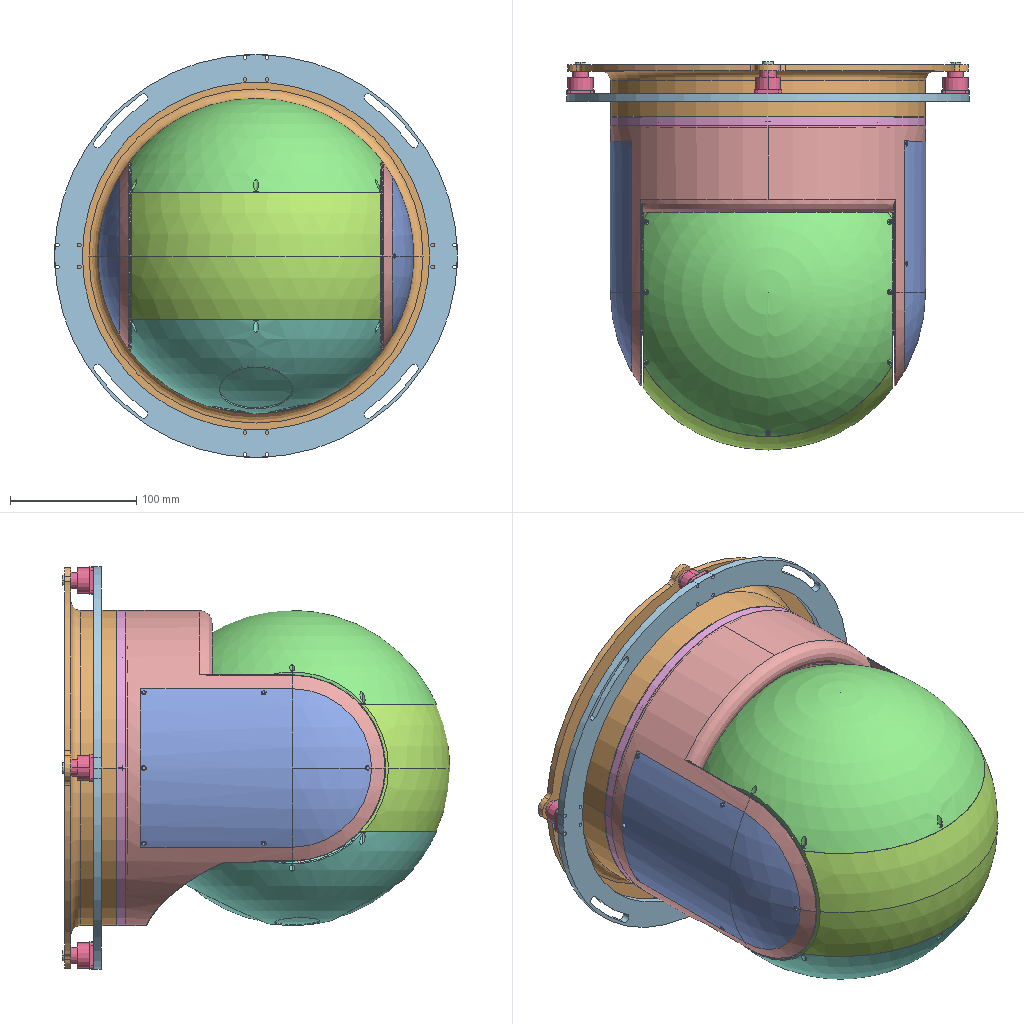Assembly | SolidWorks | 31 different items | 42 placed | box 319 x 308 x 319 mm
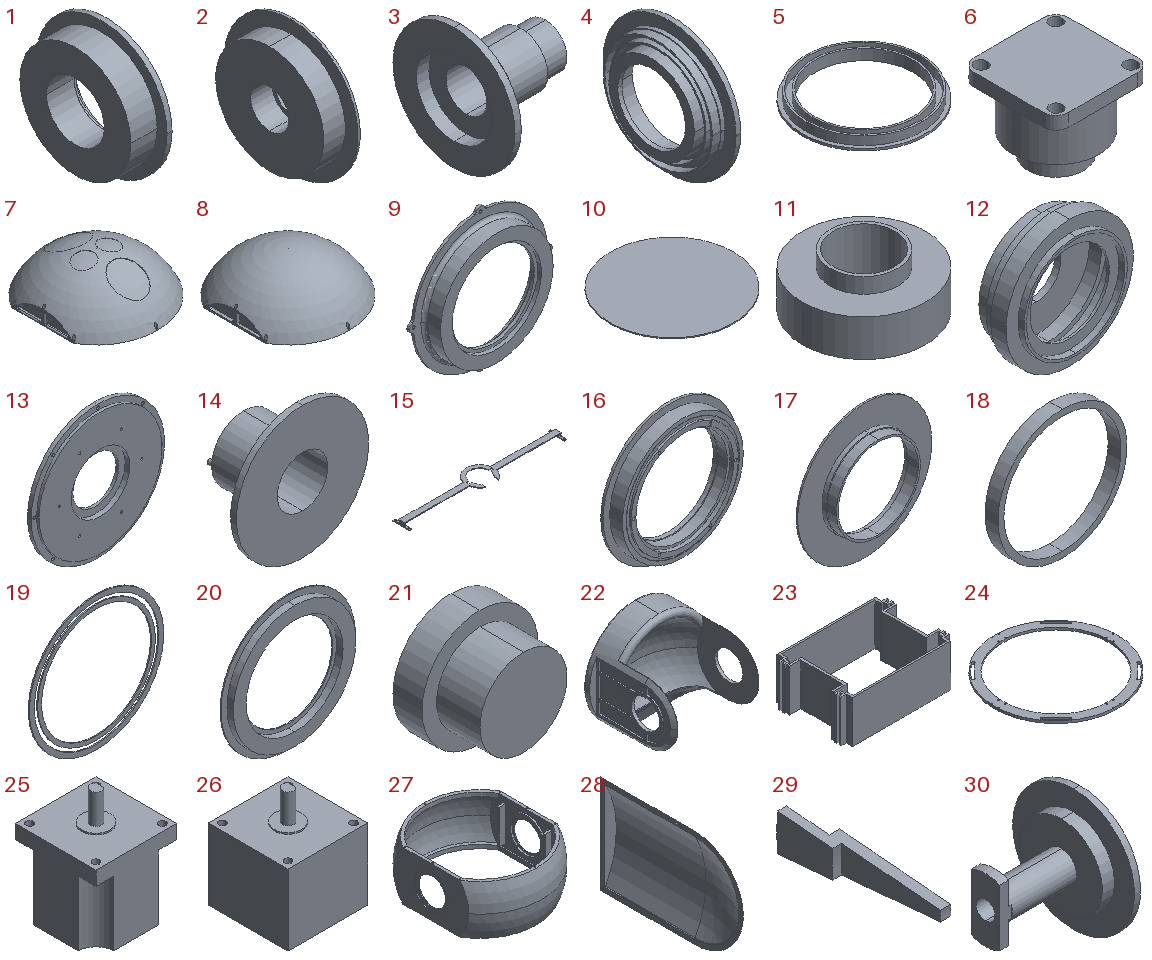Parts list (item | quantity | size | volume | features):
1 | x2 | 21.418 x 78.909 x 78.909 mm | 50880 mm3 | features Revolution 1
2 | x1 | 11.085 x 60.752 x 60.752 mm | 17812 mm3 | features Revolution 1
3 | x1 | 36.357 x 48.558 x 48.558 mm | 9786 mm3 | features Revolution 1
4 | x2 | 14.383 x 84 x 84 mm | 20141 mm3 | features ICE 1, Revolution 1
5 | x2 | 69 x 69 x 6 mm | 3446 mm3 | features Extrusion 1, ICE 1
6 | x4 | 22 x 22 x 18 mm | 5008 mm3 | features ICE 2, Cut 1, Extrusion 1, Fillet 1
7 | x1 | 198 x 229.129 x 75 mm | 126524 mm3 | features ICE 7, Fillet 2, Cut 1, MirrorPattern 1, OffsetRefSurface 1, Revolution 1, Shell 1
8 | x1 | 198 x 229.129 x 75 mm | 135832 mm3 | features ICE 5, Cut 1, Fillet 1, MirrorPattern 1, Revolution 1, Shell 1
9 | x1 | 317.492 x 41 x 317.492 mm | 402589 mm3 | features Cut 2, Fillet 2, ICE 2, Revolution 1
10 | x1 | 254 x 254 x 2 mm | 101341 mm3 | features Extrusion 1
11 | x1 | 40 x 40 x 17 mm | 11640 mm3 | features Extrusion 1, ICE 1
12 | x1 | 106 x 37.5 x 106 mm | 44844 mm3 | features Revolution 1
13 | x1 | 250 x 14 x 250 mm | 269051 mm3 | features Cut 3, Revolution 1
14 | x1 | 80.737 x 39 x 80.737 mm | 34067 mm3 | features ICE 1, Revolution 1
15 | x1 | 236.176 x 39.297 x 6 mm | 2428 mm3 | features ICE 2, Extrusion 1
16 | x1 | 204 x 26 x 204 mm | 266673 mm3 | features ICE 2, Revolution 1
17 | x1 | 204 x 23.032 x 204 mm | 75722 mm3 | features Revolution 1
18 | x1 | 140.991 x 14 x 140.991 mm | 38449 mm3 | features Revolution 1
19 | x1 | 148.991 x 1.185 x 148.991 mm | 4958 mm3 | features Revolution 1
20 | x1 | 138.727 x 7.789 x 138.727 mm | 36485 mm3 | features Revolution 1
21 | x4 | 8 x 5 x 8 mm | 185.354 mm3 | features Revolution 1
22 | x1 | 250 x 205.985 x 250 mm | 931758 mm3 | features Fillet 16, Cut 11, ICE 3, MirrorPattern 2, PlanarSurface 2, CirPattern 1, NetBlend 1, RevCut 1, Revolution 1, SewRefSurface 1, SurfCut 1
23 | x1 | 180 x 125.252 x 70 mm | 170034 mm3 | features Extrusion 1
24 | x1 | 319.492 x 319.492 x 6 mm | 113822 mm3 | features Extrusion 1
25 | x1 | 57 x 57 x 78 mm | 159872 mm3 | features ICE 5, Extrusion 1
26 | x1 | 57 x 57 x 73 mm | 162987 mm3 | features ICE 4, Extrusion 1
27 | x1 | 198 x 250 x 100 mm | 273792 mm3 | features ICE 7, Cut 4, MirrorPattern 2, CirPattern 1, HoleWzd 1, Revolution 1, Shell 1
28 | x2 | 17 x 182.936 x 125.873 mm | 49131 mm3 | features ICE 3, Cut 1, Fillet 1, OffsetRefSurface 1, Revolution 1, SewRefSurface 1, Shell 1
29 | x2 | 3.582 x 28.652 x 6.869 mm | 248.306 mm3 | features Revolution 1
30 | x1 | 40.262 x 52.049 x 52.049 mm | 10319 mm3 | features Cut 1, Revolution 1
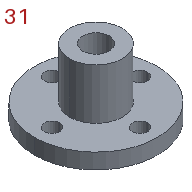31 | x1 | 28 x 28 x 15 mm | 2897 mm3 | features ICE 3, CirPattern 1, Extrusion 1
Mates (type | each side: item.copy, entity, surface, feature):
InPlace | 22.1 plane | assembly plane
InPlace | 28.1 plane | assembly plane
InPlace | 27.1 plane | assembly plane
InPlace | 13.1 plane | assembly plane
Coincident | 27.1 face plane Cut-Extrude1 | 7.1 face plane Cut-Extrude1
Coincident | 27.1 face plane Revolve1 | 7.1 face plane Revolve1
Coincident | 27.1 edge | 7.1 edge
InPlace | 9.1 plane | assembly plane
InPlace | 9.1 face plane Cut-Extrude1 | 10.1 plane
Coincident | 27.1 face plane Cut-Extrude1 | 8.1 face plane Cut-Extrude1
Coincident | 27.1 face plane Revolve1 | 8.1 face plane Revolve1
Coincident | 27.1 edge | 8.1 edge
InPlace | 9.1 face plane Revolve1 | 6.1 plane
InPlace | 6.1 face plane Boss-Extrude3 | 24.1 plane
InPlace | 16.1 plane | assembly plane
InPlace | 18.1 plane | assembly plane
InPlace | 17.1 plane | assembly plane
InPlace | 19.1 plane | assembly plane
InPlace | 12.1 plane | assembly plane
InPlace | 20.1 plane | assembly plane
InPlace | 14.1 plane | assembly plane
InPlace | 14.1 face plane Boss-Extrude1 | 15.1 plane
InPlace | 4.1 plane | assembly plane
InPlace | 1.1 plane | assembly plane
InPlace | 3.1 plane | assembly plane
InPlace | 2.1 plane | assembly plane
InPlace | 30.1 plane | assembly plane
InPlace | 29.1 plane | assembly plane
InPlace | 27.1 face plane Boss-Extrude4 | 23.1 plane
InPlace | 27.1 face plane Cut-Extrude6 | 5.1 plane
Coincident | 9.1 face plane Revolve1 | 21.1 face plane Revolve1
Concentric | 9.1 face cylinder Cut-Extrude2 | 21.1 face cylinder Revolve1
Coincident | 23.1 face plane Boss-Extrude1 | 25.1 face plane Boss-Extrude1 | 2 times
DistanceDim | 25.1 face plane Boss-Extrude1 | 23.1 face plane Boss-Extrude1
Coincident | 23.1 face plane Boss-Extrude1 | 11.1 face plane Boss-Extrude1
Concentric | 1.2 face cylinder Revolve1 | 11.1 face cylinder Boss-Extrude1
Coincident | 23.1 face plane Boss-Extrude1 | 31.1 face plane Boss-Extrude1
Concentric | 1.1 face cylinder Revolve1 | 31.1 face cylinder Boss-Extrude1
Coincident | 23.1 face plane Boss-Extrude1 | 26.1 face plane Boss-Extrude1
Coincident | 25.1 face plane Boss-Extrude1 | 26.1 face plane Boss-Extrude1 | 2 times